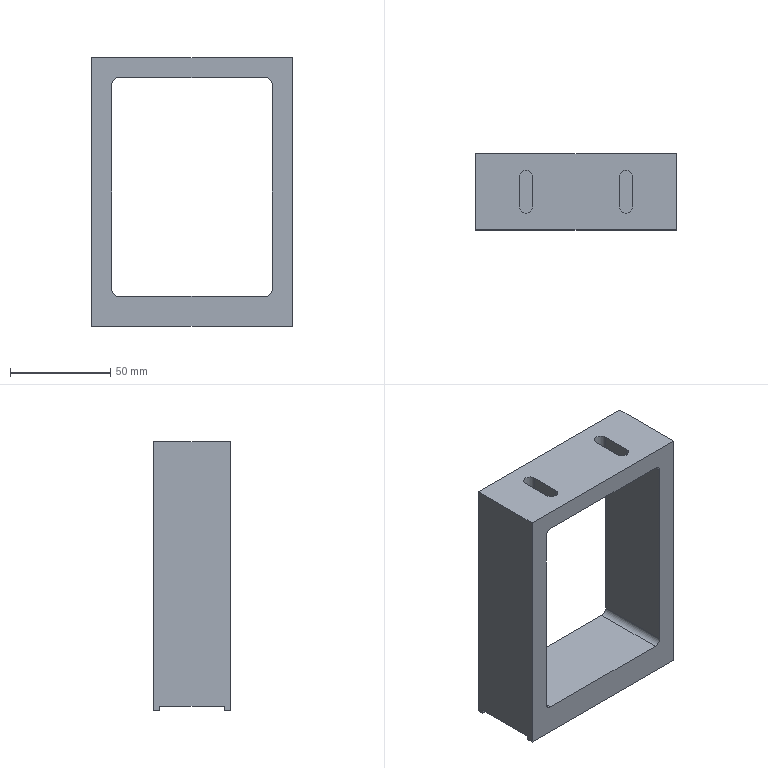Part | NX | features BREP 1 | 1 solid | 42 faces | box 100 x 38 x 134 mm | volume 168763 mm3 | plane 18 | cylinder 16 | cone 8 | commonest cylinder face diameters 3.3 x8 6 x4 6.5 x4
STEP:
#1=CARTESIAN_POINT('',(-38.35,11.,12.1));
#2=VERTEX_POINT('',#1);
#3=CARTESIAN_POINT('',(-41.65,11.,12.1));
#4=VERTEX_POINT('',#3);
#5=CARTESIAN_POINT('',(-40.,11.,12.1));
#6=DIRECTION('',(0.,0.,-1.));
#7=DIRECTION('',(-1.,0.,0.));
#8=AXIS2_PLACEMENT_3D('',#5,#6,#7);
#9=CIRCLE('',#8,1.65);
#10=EDGE_CURVE('',#2,#4,#9,.T.);
#11=ORIENTED_EDGE('',*,*,#10,.F.);
#12=CARTESIAN_POINT('',(-38.35,11.,2.));
#13=VERTEX_POINT('',#12);
#14=CARTESIAN_POINT('',(-38.35,11.,2.));
#15=DIRECTION('',(0.,0.,-1.));
#16=VECTOR('',#15,1000.);
#17=LINE('',#14,#16);
#18=EDGE_CURVE('',#2,#13,#17,.T.);
#19=ORIENTED_EDGE('',*,*,#18,.T.);
#20=CARTESIAN_POINT('',(-41.65,11.,2.));
#21=VERTEX_POINT('',#20);
#22=CARTESIAN_POINT('',(-40.,11.,2.));
#23=DIRECTION('',(0.,0.,-1.));
#24=DIRECTION('',(-1.,0.,0.));
#25=AXIS2_PLACEMENT_3D('',#22,#23,#24);
#26=CIRCLE('',#25,1.65);
#27=EDGE_CURVE('',#13,#21,#26,.T.);
#28=ORIENTED_EDGE('',*,*,#27,.T.);
#29=CARTESIAN_POINT('',(-41.65,11.,2.));
#30=DIRECTION('',(0.,0.,-1.));
#31=VECTOR('',#30,1000.);
#32=LINE('',#29,#31);
#33=EDGE_CURVE('',#4,#21,#32,.T.);
#34=ORIENTED_EDGE('',*,*,#33,.F.);
#35=EDGE_LOOP('',(#11,#19,#28,#34));
#36=FACE_BOUND('',#35,.T.);
#37=CARTESIAN_POINT('',(-40.,11.,2.));
#38=DIRECTION('',(0.,0.,-1.));
#39=DIRECTION('',(-1.,0.,0.));
#40=AXIS2_PLACEMENT_3D('',#37,#38,#39);
#41=CYLINDRICAL_SURFACE('',#40,1.65);
#42=ADVANCED_FACE('',(#36),#41,.F.);
#43=CARTESIAN_POINT('',(-40.,11.,13.091));
#44=VERTEX_POINT('',#43);
#45=CARTESIAN_POINT('',(-41.65,11.,12.1));
#46=DIRECTION('',(-0.8572,0.,-0.515));
#47=VECTOR('',#46,1000.);
#48=LINE('',#45,#47);
#49=EDGE_CURVE('',#44,#4,#48,.T.);
#50=ORIENTED_EDGE('',*,*,#49,.F.);
#51=CARTESIAN_POINT('',(-38.35,11.,12.1));
#52=DIRECTION('',(0.8572,0.,-0.515));
#53=VECTOR('',#52,1000.);
#54=LINE('',#51,#53);
#55=EDGE_CURVE('',#44,#2,#54,.T.);
#56=ORIENTED_EDGE('',*,*,#55,.T.);
#57=ORIENTED_EDGE('',*,*,#10,.T.);
#58=EDGE_LOOP('',(#50,#56,#57));
#59=FACE_BOUND('',#58,.T.);
#60=CARTESIAN_POINT('',(-40.,11.,12.1));
#61=DIRECTION('',(0.,0.,-1.));
#62=DIRECTION('',(-1.,0.,0.));
#63=AXIS2_PLACEMENT_3D('',#60,#61,#62);
#64=CONICAL_SURFACE('',#63,1.65,1.03);
#65=ADVANCED_FACE('',(#59),#64,.F.);
#66=CARTESIAN_POINT('',(-38.35,-11.,12.1));
#67=VERTEX_POINT('',#66);
#68=CARTESIAN_POINT('',(-41.65,-11.,12.1));
#69=VERTEX_POINT('',#68);
#70=CARTESIAN_POINT('',(-40.,-11.,12.1));
#71=DIRECTION('',(0.,0.,-1.));
#72=DIRECTION('',(-1.,0.,0.));
#73=AXIS2_PLACEMENT_3D('',#70,#71,#72);
#74=CIRCLE('',#73,1.65);
#75=EDGE_CURVE('',#67,#69,#74,.T.);
#76=ORIENTED_EDGE('',*,*,#75,.F.);
#77=CARTESIAN_POINT('',(-38.35,-11.,2.));
#78=VERTEX_POINT('',#77);
#79=CARTESIAN_POINT('',(-38.35,-11.,2.));
#80=DIRECTION('',(0.,0.,-1.));
#81=VECTOR('',#80,1000.);
#82=LINE('',#79,#81);
#83=EDGE_CURVE('',#67,#78,#82,.T.);
#84=ORIENTED_EDGE('',*,*,#83,.T.);
#85=CARTESIAN_POINT('',(-41.65,-11.,2.));
#86=VERTEX_POINT('',#85);
#87=CARTESIAN_POINT('',(-40.,-11.,2.));
#88=DIRECTION('',(0.,0.,-1.));
#89=DIRECTION('',(-1.,0.,0.));
#90=AXIS2_PLACEMENT_3D('',#87,#88,#89);
#91=CIRCLE('',#90,1.65);
#92=EDGE_CURVE('',#78,#86,#91,.T.);
#93=ORIENTED_EDGE('',*,*,#92,.T.);
#94=CARTESIAN_POINT('',(-41.65,-11.,2.));
#95=DIRECTION('',(0.,0.,-1.));
#96=VECTOR('',#95,1000.);
#97=LINE('',#94,#96);
#98=EDGE_CURVE('',#69,#86,#97,.T.);
#99=ORIENTED_EDGE('',*,*,#98,.F.);
#100=EDGE_LOOP('',(#76,#84,#93,#99));
#101=FACE_BOUND('',#100,.T.);
#102=CARTESIAN_POINT('',(-40.,-11.,2.));
#103=DIRECTION('',(0.,0.,-1.));
#104=DIRECTION('',(-1.,0.,0.));
#105=AXIS2_PLACEMENT_3D('',#102,#103,#104);
#106=CYLINDRICAL_SURFACE('',#105,1.65);
#107=ADVANCED_FACE('',(#101),#106,.F.);
#108=CARTESIAN_POINT('',(-40.,-11.,13.091));
#109=VERTEX_POINT('',#108);
#110=CARTESIAN_POINT('',(-41.65,-11.,12.1));
#111=DIRECTION('',(-0.8572,0.,-0.515));
#112=VECTOR('',#111,1000.);
#113=LINE('',#110,#112);
#114=EDGE_CURVE('',#109,#69,#113,.T.);
#115=ORIENTED_EDGE('',*,*,#114,.F.);
#116=CARTESIAN_POINT('',(-38.35,-11.,12.1));
#117=DIRECTION('',(0.8572,0.,-0.515));
#118=VECTOR('',#117,1000.);
#119=LINE('',#116,#118);
#120=EDGE_CURVE('',#109,#67,#119,.T.);
#121=ORIENTED_EDGE('',*,*,#120,.T.);
#122=ORIENTED_EDGE('',*,*,#75,.T.);
#123=EDGE_LOOP('',(#115,#121,#122));
#124=FACE_BOUND('',#123,.T.);
#125=CARTESIAN_POINT('',(-40.,-11.,12.1));
#126=DIRECTION('',(0.,0.,-1.));
#127=DIRECTION('',(-1.,0.,0.));
#128=AXIS2_PLACEMENT_3D('',#125,#126,#127);
#129=CONICAL_SURFACE('',#128,1.65,1.03);
#130=ADVANCED_FACE('',(#124),#129,.F.);
#131=CARTESIAN_POINT('',(41.65,11.,12.1));
#132=VERTEX_POINT('',#131);
#133=CARTESIAN_POINT('',(38.35,11.,12.1));
#134=VERTEX_POINT('',#133);
#135=CARTESIAN_POINT('',(40.,11.,12.1));
#136=DIRECTION('',(0.,0.,-1.));
#137=DIRECTION('',(-1.,0.,0.));
#138=AXIS2_PLACEMENT_3D('',#135,#136,#137);
#139=CIRCLE('',#138,1.65);
#140=EDGE_CURVE('',#132,#134,#139,.T.);
#141=ORIENTED_EDGE('',*,*,#140,.F.);
#142=CARTESIAN_POINT('',(41.65,11.,2.));
#143=VERTEX_POINT('',#142);
#144=CARTESIAN_POINT('',(41.65,11.,2.));
#145=DIRECTION('',(0.,0.,-1.));
#146=VECTOR('',#145,1000.);
#147=LINE('',#144,#146);
#148=EDGE_CURVE('',#132,#143,#147,.T.);
#149=ORIENTED_EDGE('',*,*,#148,.T.);
#150=CARTESIAN_POINT('',(38.35,11.,2.));
#151=VERTEX_POINT('',#150);
#152=CARTESIAN_POINT('',(40.,11.,2.));
#153=DIRECTION('',(0.,0.,-1.));
#154=DIRECTION('',(-1.,0.,0.));
#155=AXIS2_PLACEMENT_3D('',#152,#153,#154);
#156=CIRCLE('',#155,1.65);
#157=EDGE_CURVE('',#143,#151,#156,.T.);
#158=ORIENTED_EDGE('',*,*,#157,.T.);
#159=CARTESIAN_POINT('',(38.35,11.,2.));
#160=DIRECTION('',(0.,0.,-1.));
#161=VECTOR('',#160,1000.);
#162=LINE('',#159,#161);
#163=EDGE_CURVE('',#134,#151,#162,.T.);
#164=ORIENTED_EDGE('',*,*,#163,.F.);
#165=EDGE_LOOP('',(#141,#149,#158,#164));
#166=FACE_BOUND('',#165,.T.);
#167=CARTESIAN_POINT('',(40.,11.,2.));
#168=DIRECTION('',(0.,0.,-1.));
#169=DIRECTION('',(-1.,0.,0.));
#170=AXIS2_PLACEMENT_3D('',#167,#168,#169);
#171=CYLINDRICAL_SURFACE('',#170,1.65);
#172=ADVANCED_FACE('',(#166),#171,.F.);
#173=CARTESIAN_POINT('',(40.,11.,13.091));
#174=VERTEX_POINT('',#173);
#175=CARTESIAN_POINT('',(38.35,11.,12.1));
#176=DIRECTION('',(-0.8572,0.,-0.515));
#177=VECTOR('',#176,1000.);
#178=LINE('',#175,#177);
#179=EDGE_CURVE('',#174,#134,#178,.T.);
#180=ORIENTED_EDGE('',*,*,#179,.F.);
#181=CARTESIAN_POINT('',(41.65,11.,12.1));
#182=DIRECTION('',(0.8572,0.,-0.515));
#183=VECTOR('',#182,1000.);
#184=LINE('',#181,#183);
#185=EDGE_CURVE('',#174,#132,#184,.T.);
#186=ORIENTED_EDGE('',*,*,#185,.T.);
#187=ORIENTED_EDGE('',*,*,#140,.T.);
#188=EDGE_LOOP('',(#180,#186,#187));
#189=FACE_BOUND('',#188,.T.);
#190=CARTESIAN_POINT('',(40.,11.,12.1));
#191=DIRECTION('',(0.,0.,-1.));
#192=DIRECTION('',(-1.,0.,0.));
#193=AXIS2_PLACEMENT_3D('',#190,#191,#192);
#194=CONICAL_SURFACE('',#193,1.65,1.03);
#195=ADVANCED_FACE('',(#189),#194,.F.);
#196=CARTESIAN_POINT('',(41.65,-11.,12.1));
#197=VERTEX_POINT('',#196);
#198=CARTESIAN_POINT('',(38.35,-11.,12.1));
#199=VERTEX_POINT('',#198);
#200=CARTESIAN_POINT('',(40.,-11.,12.1));
#201=DIRECTION('',(0.,0.,-1.));
#202=DIRECTION('',(-1.,0.,0.));
#203=AXIS2_PLACEMENT_3D('',#200,#201,#202);
#204=CIRCLE('',#203,1.65);
#205=EDGE_CURVE('',#197,#199,#204,.T.);
#206=ORIENTED_EDGE('',*,*,#205,.F.);
#207=CARTESIAN_POINT('',(41.65,-11.,2.));
#208=VERTEX_POINT('',#207);
#209=CARTESIAN_POINT('',(41.65,-11.,2.));
#210=DIRECTION('',(0.,0.,-1.));
#211=VECTOR('',#210,1000.);
#212=LINE('',#209,#211);
#213=EDGE_CURVE('',#197,#208,#212,.T.);
#214=ORIENTED_EDGE('',*,*,#213,.T.);
#215=CARTESIAN_POINT('',(38.35,-11.,2.));
#216=VERTEX_POINT('',#215);
#217=CARTESIAN_POINT('',(40.,-11.,2.));
#218=DIRECTION('',(0.,0.,-1.));
#219=DIRECTION('',(-1.,0.,0.));
#220=AXIS2_PLACEMENT_3D('',#217,#218,#219);
#221=CIRCLE('',#220,1.65);
#222=EDGE_CURVE('',#208,#216,#221,.T.);
#223=ORIENTED_EDGE('',*,*,#222,.T.);
#224=CARTESIAN_POINT('',(38.35,-11.,2.));
#225=DIRECTION('',(0.,0.,-1.));
#226=VECTOR('',#225,1000.);
#227=LINE('',#224,#226);
#228=EDGE_CURVE('',#199,#216,#227,.T.);
#229=ORIENTED_EDGE('',*,*,#228,.F.);
#230=EDGE_LOOP('',(#206,#214,#223,#229));
#231=FACE_BOUND('',#230,.T.);
#232=CARTESIAN_POINT('',(40.,-11.,2.));
#233=DIRECTION('',(0.,0.,-1.));
#234=DIRECTION('',(-1.,0.,0.));
#235=AXIS2_PLACEMENT_3D('',#232,#233,#234);
#236=CYLINDRICAL_SURFACE('',#235,1.65);
#237=ADVANCED_FACE('',(#231),#236,.F.);
#238=CARTESIAN_POINT('',(40.,-11.,13.091));
#239=VERTEX_POINT('',#238);
#240=CARTESIAN_POINT('',(38.35,-11.,12.1));
#241=DIRECTION('',(-0.8572,0.,-0.515));
#242=VECTOR('',#241,1000.);
#243=LINE('',#240,#242);
#244=EDGE_CURVE('',#239,#199,#243,.T.);
#245=ORIENTED_EDGE('',*,*,#244,.F.);
#246=CARTESIAN_POINT('',(41.65,-11.,12.1));
#247=DIRECTION('',(0.8572,0.,-0.515));
#248=VECTOR('',#247,1000.);
#249=LINE('',#246,#248);
#250=EDGE_CURVE('',#239,#197,#249,.T.);
#251=ORIENTED_EDGE('',*,*,#250,.T.);
#252=ORIENTED_EDGE('',*,*,#205,.T.);
#253=EDGE_LOOP('',(#245,#251,#252));
#254=FACE_BOUND('',#253,.T.);
#255=CARTESIAN_POINT('',(40.,-11.,12.1));
#256=DIRECTION('',(0.,0.,-1.));
#257=DIRECTION('',(-1.,0.,0.));
#258=AXIS2_PLACEMENT_3D('',#255,#256,#257);
#259=CONICAL_SURFACE('',#258,1.65,1.03);
#260=ADVANCED_FACE('',(#254),#259,.F.);
#261=CARTESIAN_POINT('',(-50.,16.,0.));
#262=VERTEX_POINT('',#261);
#263=CARTESIAN_POINT('',(50.,16.,0.));
#264=VERTEX_POINT('',#263);
#265=CARTESIAN_POINT('',(0.,16.,0.));
#266=DIRECTION('',(1.,0.,0.));
#267=VECTOR('',#266,1000.);
#268=LINE('',#265,#267);
#269=EDGE_CURVE('',#262,#264,#268,.T.);
#270=ORIENTED_EDGE('',*,*,#269,.F.);
#271=CARTESIAN_POINT('',(-50.,19.,0.));
#272=VERTEX_POINT('',#271);
#273=CARTESIAN_POINT('',(-50.,-19.,0.));
#274=DIRECTION('',(0.,-1.,0.));
#275=VECTOR('',#274,1000.);
#276=LINE('',#273,#275);
#277=EDGE_CURVE('',#272,#262,#276,.T.);
#278=ORIENTED_EDGE('',*,*,#277,.F.);
#279=CARTESIAN_POINT('',(50.,19.,0.));
#280=VERTEX_POINT('',#279);
#281=CARTESIAN_POINT('',(-50.,19.,0.));
#282=DIRECTION('',(-1.,0.,0.));
#283=VECTOR('',#282,1000.);
#284=LINE('',#281,#283);
#285=EDGE_CURVE('',#280,#272,#284,.T.);
#286=ORIENTED_EDGE('',*,*,#285,.F.);
#287=CARTESIAN_POINT('',(50.,-19.,0.));
#288=DIRECTION('',(0.,1.,0.));
#289=VECTOR('',#288,1000.);
#290=LINE('',#287,#289);
#291=EDGE_CURVE('',#264,#280,#290,.T.);
#292=ORIENTED_EDGE('',*,*,#291,.F.);
#293=EDGE_LOOP('',(#270,#278,#286,#292));
#294=FACE_BOUND('',#293,.T.);
#295=CARTESIAN_POINT('',(0.,0.,0.));
#296=DIRECTION('',(0.,0.,-1.));
#297=DIRECTION('',(0.,-1.,0.));
#298=AXIS2_PLACEMENT_3D('',#295,#296,#297);
#299=PLANE('',#298);
#300=ADVANCED_FACE('',(#294),#299,.T.);
#301=CARTESIAN_POINT('',(50.,16.,2.));
#302=VERTEX_POINT('',#301);
#303=CARTESIAN_POINT('',(50.,-16.,2.));
#304=VERTEX_POINT('',#303);
#305=CARTESIAN_POINT('',(50.,-19.,2.));
#306=DIRECTION('',(0.,-1.,0.));
#307=VECTOR('',#306,1000.);
#308=LINE('',#305,#307);
#309=EDGE_CURVE('',#302,#304,#308,.T.);
#310=ORIENTED_EDGE('',*,*,#309,.F.);
#311=CARTESIAN_POINT('',(50.,16.,134.));
#312=DIRECTION('',(0.,0.,-1.));
#313=VECTOR('',#312,1000.);
#314=LINE('',#311,#313);
#315=EDGE_CURVE('',#302,#264,#314,.T.);
#316=ORIENTED_EDGE('',*,*,#315,.T.);
#317=ORIENTED_EDGE('',*,*,#291,.T.);
#318=CARTESIAN_POINT('',(50.,19.,134.));
#319=VERTEX_POINT('',#318);
#320=CARTESIAN_POINT('',(50.,19.,134.));
#321=DIRECTION('',(0.,0.,-1.));
#322=VECTOR('',#321,1000.);
#323=LINE('',#320,#322);
#324=EDGE_CURVE('',#319,#280,#323,.T.);
#325=ORIENTED_EDGE('',*,*,#324,.F.);
#326=CARTESIAN_POINT('',(50.,-19.,134.));
#327=VERTEX_POINT('',#326);
#328=CARTESIAN_POINT('',(50.,-19.,134.));
#329=DIRECTION('',(0.,1.,0.));
#330=VECTOR('',#329,1000.);
#331=LINE('',#328,#330);
#332=EDGE_CURVE('',#327,#319,#331,.T.);
#333=ORIENTED_EDGE('',*,*,#332,.F.);
#334=CARTESIAN_POINT('',(50.,-19.,0.));
#335=VERTEX_POINT('',#334);
#336=CARTESIAN_POINT('',(50.,-19.,134.));
#337=DIRECTION('',(0.,0.,-1.));
#338=VECTOR('',#337,1000.);
#339=LINE('',#336,#338);
#340=EDGE_CURVE('',#327,#335,#339,.T.);
#341=ORIENTED_EDGE('',*,*,#340,.T.);
#342=CARTESIAN_POINT('',(50.,-16.,0.));
#343=VERTEX_POINT('',#342);
#344=CARTESIAN_POINT('',(50.,-19.,0.));
#345=DIRECTION('',(0.,1.,0.));
#346=VECTOR('',#345,1000.);
#347=LINE('',#344,#346);
#348=EDGE_CURVE('',#335,#343,#347,.T.);
#349=ORIENTED_EDGE('',*,*,#348,.T.);
#350=CARTESIAN_POINT('',(50.,-16.,134.));
#351=DIRECTION('',(0.,0.,1.));
#352=VECTOR('',#351,1000.);
#353=LINE('',#350,#352);
#354=EDGE_CURVE('',#343,#304,#353,.T.);
#355=ORIENTED_EDGE('',*,*,#354,.T.);
#356=EDGE_LOOP('',(#310,#316,#317,#325,#333,#341,#349,#355));
#357=FACE_BOUND('',#356,.T.);
#358=CARTESIAN_POINT('',(50.,-19.,134.));
#359=DIRECTION('',(-1.,0.,0.));
#360=DIRECTION('',(0.,0.,1.));
#361=AXIS2_PLACEMENT_3D('',#358,#359,#360);
#362=PLANE('',#361);
#363=ADVANCED_FACE('',(#357),#362,.F.);
#364=ORIENTED_EDGE('',*,*,#285,.T.);
#365=CARTESIAN_POINT('',(-50.,19.,134.));
#366=VERTEX_POINT('',#365);
#367=CARTESIAN_POINT('',(-50.,19.,134.));
#368=DIRECTION('',(0.,0.,-1.));
#369=VECTOR('',#368,1000.);
#370=LINE('',#367,#369);
#371=EDGE_CURVE('',#366,#272,#370,.T.);
#372=ORIENTED_EDGE('',*,*,#371,.F.);
#373=CARTESIAN_POINT('',(-50.,19.,134.));
#374=DIRECTION('',(-1.,0.,0.));
#375=VECTOR('',#374,1000.);
#376=LINE('',#373,#375);
#377=EDGE_CURVE('',#319,#366,#376,.T.);
#378=ORIENTED_EDGE('',*,*,#377,.F.);
#379=ORIENTED_EDGE('',*,*,#324,.T.);
#380=EDGE_LOOP('',(#364,#372,#378,#379));
#381=FACE_BOUND('',#380,.T.);
#382=CARTESIAN_POINT('',(40.,19.,18.));
#383=VERTEX_POINT('',#382);
#384=CARTESIAN_POINT('',(40.,19.,121.));
#385=VERTEX_POINT('',#384);
#386=CARTESIAN_POINT('',(40.,19.,124.));
#387=DIRECTION('',(0.,0.,1.));
#388=VECTOR('',#387,1000.);
#389=LINE('',#386,#388);
#390=EDGE_CURVE('',#383,#385,#389,.T.);
#391=ORIENTED_EDGE('',*,*,#390,.T.);
#392=CARTESIAN_POINT('',(37.,19.,124.));
#393=VERTEX_POINT('',#392);
#394=CARTESIAN_POINT('',(37.,19.,121.));
#395=DIRECTION('',(0.,-1.,0.));
#396=DIRECTION('',(0.,0.,-1.));
#397=AXIS2_PLACEMENT_3D('',#394,#395,#396);
#398=CIRCLE('',#397,3.);
#399=EDGE_CURVE('',#385,#393,#398,.T.);
#400=ORIENTED_EDGE('',*,*,#399,.T.);
#401=CARTESIAN_POINT('',(-37.,19.,124.));
#402=VERTEX_POINT('',#401);
#403=CARTESIAN_POINT('',(40.,19.,124.));
#404=DIRECTION('',(-1.,0.,0.));
#405=VECTOR('',#404,1000.);
#406=LINE('',#403,#405);
#407=EDGE_CURVE('',#393,#402,#406,.T.);
#408=ORIENTED_EDGE('',*,*,#407,.T.);
#409=CARTESIAN_POINT('',(-40.,19.,121.));
#410=VERTEX_POINT('',#409);
#411=CARTESIAN_POINT('',(-37.,19.,121.));
#412=DIRECTION('',(0.,-1.,0.));
#413=DIRECTION('',(0.,0.,-1.));
#414=AXIS2_PLACEMENT_3D('',#411,#412,#413);
#415=CIRCLE('',#414,3.);
#416=EDGE_CURVE('',#402,#410,#415,.T.);
#417=ORIENTED_EDGE('',*,*,#416,.T.);
#418=CARTESIAN_POINT('',(-40.,19.,18.));
#419=VERTEX_POINT('',#418);
#420=CARTESIAN_POINT('',(-40.,19.,124.));
#421=DIRECTION('',(0.,0.,-1.));
#422=VECTOR('',#421,1000.);
#423=LINE('',#420,#422);
#424=EDGE_CURVE('',#410,#419,#423,.T.);
#425=ORIENTED_EDGE('',*,*,#424,.T.);
#426=CARTESIAN_POINT('',(-37.,19.,15.));
#427=VERTEX_POINT('',#426);
#428=CARTESIAN_POINT('',(-37.,19.,18.));
#429=DIRECTION('',(0.,-1.,0.));
#430=DIRECTION('',(0.,0.,-1.));
#431=AXIS2_PLACEMENT_3D('',#428,#429,#430);
#432=CIRCLE('',#431,3.);
#433=EDGE_CURVE('',#419,#427,#432,.T.);
#434=ORIENTED_EDGE('',*,*,#433,.T.);
#435=CARTESIAN_POINT('',(37.,19.,15.));
#436=VERTEX_POINT('',#435);
#437=CARTESIAN_POINT('',(40.,19.,15.));
#438=DIRECTION('',(1.,0.,0.));
#439=VECTOR('',#438,1000.);
#440=LINE('',#437,#439);
#441=EDGE_CURVE('',#427,#436,#440,.T.);
#442=ORIENTED_EDGE('',*,*,#441,.T.);
#443=CARTESIAN_POINT('',(37.,19.,18.));
#444=DIRECTION('',(0.,-1.,0.));
#445=DIRECTION('',(0.,0.,-1.));
#446=AXIS2_PLACEMENT_3D('',#443,#444,#445);
#447=CIRCLE('',#446,3.);
#448=EDGE_CURVE('',#436,#383,#447,.T.);
#449=ORIENTED_EDGE('',*,*,#448,.T.);
#450=EDGE_LOOP('',(#391,#400,#408,#417,#425,#434,#442,#449));
#451=FACE_BOUND('',#450,.T.);
#452=CARTESIAN_POINT('',(-50.,19.,134.));
#453=DIRECTION('',(0.,-1.,0.));
#454=DIRECTION('',(0.,0.,-1.));
#455=AXIS2_PLACEMENT_3D('',#452,#453,#454);
#456=PLANE('',#455);
#457=ADVANCED_FACE('',(#381,#451),#456,.F.);
#458=ORIENTED_EDGE('',*,*,#277,.T.);
#459=CARTESIAN_POINT('',(-50.,16.,2.));
#460=VERTEX_POINT('',#459);
#461=CARTESIAN_POINT('',(-50.,16.,134.));
#462=DIRECTION('',(0.,0.,1.));
#463=VECTOR('',#462,1000.);
#464=LINE('',#461,#463);
#465=EDGE_CURVE('',#262,#460,#464,.T.);
#466=ORIENTED_EDGE('',*,*,#465,.T.);
#467=CARTESIAN_POINT('',(-50.,-16.,2.));
#468=VERTEX_POINT('',#467);
#469=CARTESIAN_POINT('',(-50.,-19.,2.));
#470=DIRECTION('',(0.,1.,0.));
#471=VECTOR('',#470,1000.);
#472=LINE('',#469,#471);
#473=EDGE_CURVE('',#468,#460,#472,.T.);
#474=ORIENTED_EDGE('',*,*,#473,.F.);
#475=CARTESIAN_POINT('',(-50.,-16.,0.));
#476=VERTEX_POINT('',#475);
#477=CARTESIAN_POINT('',(-50.,-16.,134.));
#478=DIRECTION('',(0.,0.,-1.));
#479=VECTOR('',#478,1000.);
#480=LINE('',#477,#479);
#481=EDGE_CURVE('',#468,#476,#480,.T.);
#482=ORIENTED_EDGE('',*,*,#481,.T.);
#483=CARTESIAN_POINT('',(-50.,-19.,0.));
#484=VERTEX_POINT('',#483);
#485=CARTESIAN_POINT('',(-50.,-19.,0.));
#486=DIRECTION('',(0.,-1.,0.));
#487=VECTOR('',#486,1000.);
#488=LINE('',#485,#487);
#489=EDGE_CURVE('',#476,#484,#488,.T.);
#490=ORIENTED_EDGE('',*,*,#489,.T.);
#491=CARTESIAN_POINT('',(-50.,-19.,134.));
#492=VERTEX_POINT('',#491);
#493=CARTESIAN_POINT('',(-50.,-19.,134.));
#494=DIRECTION('',(0.,0.,-1.));
#495=VECTOR('',#494,1000.);
#496=LINE('',#493,#495);
#497=EDGE_CURVE('',#492,#484,#496,.T.);
#498=ORIENTED_EDGE('',*,*,#497,.F.);
#499=CARTESIAN_POINT('',(-50.,-19.,134.));
#500=DIRECTION('',(0.,-1.,0.));
#501=VECTOR('',#500,1000.);
#502=LINE('',#499,#501);
#503=EDGE_CURVE('',#366,#492,#502,.T.);
#504=ORIENTED_EDGE('',*,*,#503,.F.);
#505=ORIENTED_EDGE('',*,*,#371,.T.);
#506=EDGE_LOOP('',(#458,#466,#474,#482,#490,#498,#504,#505));
#507=FACE_BOUND('',#506,.T.);
#508=CARTESIAN_POINT('',(-50.,-19.,134.));
#509=DIRECTION('',(1.,0.,0.));
#510=DIRECTION('',(0.,1.,0.));
#511=AXIS2_PLACEMENT_3D('',#508,#509,#510);
#512=PLANE('',#511);
#513=ADVANCED_FACE('',(#507),#512,.F.);
#514=CARTESIAN_POINT('',(-50.,-19.,0.));
#515=DIRECTION('',(1.,0.,0.));
#516=VECTOR('',#515,1000.);
#517=LINE('',#514,#516);
#518=EDGE_CURVE('',#484,#335,#517,.T.);
#519=ORIENTED_EDGE('',*,*,#518,.T.);
#520=ORIENTED_EDGE('',*,*,#340,.F.);
#521=CARTESIAN_POINT('',(-50.,-19.,134.));
#522=DIRECTION('',(1.,0.,0.));
#523=VECTOR('',#522,1000.);
#524=LINE('',#521,#523);
#525=EDGE_CURVE('',#492,#327,#524,.T.);
#526=ORIENTED_EDGE('',*,*,#525,.F.);
#527=ORIENTED_EDGE('',*,*,#497,.T.);
#528=EDGE_LOOP('',(#519,#520,#526,#527));
#529=FACE_BOUND('',#528,.T.);
#530=CARTESIAN_POINT('',(-37.,-19.,15.));
#531=VERTEX_POINT('',#530);
#532=CARTESIAN_POINT('',(37.,-19.,15.));
#533=VERTEX_POINT('',#532);
#534=CARTESIAN_POINT('',(40.,-19.,15.));
#535=DIRECTION('',(1.,0.,0.));
#536=VECTOR('',#535,1000.);
#537=LINE('',#534,#536);
#538=EDGE_CURVE('',#531,#533,#537,.T.);
#539=ORIENTED_EDGE('',*,*,#538,.F.);
#540=CARTESIAN_POINT('',(-40.,-19.,18.));
#541=VERTEX_POINT('',#540);
#542=CARTESIAN_POINT('',(-37.,-19.,18.));
#543=DIRECTION('',(0.,1.,0.));
#544=DIRECTION('',(0.,0.,1.));
#545=AXIS2_PLACEMENT_3D('',#542,#543,#544);
#546=CIRCLE('',#545,3.);
#547=EDGE_CURVE('',#531,#541,#546,.T.);
#548=ORIENTED_EDGE('',*,*,#547,.T.);
#549=CARTESIAN_POINT('',(-40.,-19.,121.));
#550=VERTEX_POINT('',#549);
#551=CARTESIAN_POINT('',(-40.,-19.,124.));
#552=DIRECTION('',(0.,0.,-1.));
#553=VECTOR('',#552,1000.);
#554=LINE('',#551,#553);
#555=EDGE_CURVE('',#550,#541,#554,.T.);
#556=ORIENTED_EDGE('',*,*,#555,.F.);
#557=CARTESIAN_POINT('',(-37.,-19.,124.));
#558=VERTEX_POINT('',#557);
#559=CARTESIAN_POINT('',(-37.,-19.,121.));
#560=DIRECTION('',(0.,1.,0.));
#561=DIRECTION('',(0.,0.,1.));
#562=AXIS2_PLACEMENT_3D('',#559,#560,#561);
#563=CIRCLE('',#562,3.);
#564=EDGE_CURVE('',#550,#558,#563,.T.);
#565=ORIENTED_EDGE('',*,*,#564,.T.);
#566=CARTESIAN_POINT('',(37.,-19.,124.));
#567=VERTEX_POINT('',#566);
#568=CARTESIAN_POINT('',(40.,-19.,124.));
#569=DIRECTION('',(-1.,0.,0.));
#570=VECTOR('',#569,1000.);
#571=LINE('',#568,#570);
#572=EDGE_CURVE('',#567,#558,#571,.T.);
#573=ORIENTED_EDGE('',*,*,#572,.F.);
#574=CARTESIAN_POINT('',(40.,-19.,121.));
#575=VERTEX_POINT('',#574);
#576=CARTESIAN_POINT('',(37.,-19.,121.));
#577=DIRECTION('',(0.,1.,0.));
#578=DIRECTION('',(0.,0.,1.));
#579=AXIS2_PLACEMENT_3D('',#576,#577,#578);
#580=CIRCLE('',#579,3.);
#581=EDGE_CURVE('',#567,#575,#580,.T.);
#582=ORIENTED_EDGE('',*,*,#581,.T.);
#583=CARTESIAN_POINT('',(40.,-19.,18.));
#584=VERTEX_POINT('',#583);
#585=CARTESIAN_POINT('',(40.,-19.,124.));
#586=DIRECTION('',(0.,0.,1.));
#587=VECTOR('',#586,1000.);
#588=LINE('',#585,#587);
#589=EDGE_CURVE('',#584,#575,#588,.T.);
#590=ORIENTED_EDGE('',*,*,#589,.F.);
#591=CARTESIAN_POINT('',(37.,-19.,18.));
#592=DIRECTION('',(0.,1.,0.));
#593=DIRECTION('',(0.,0.,1.));
#594=AXIS2_PLACEMENT_3D('',#591,#592,#593);
#595=CIRCLE('',#594,3.);
#596=EDGE_CURVE('',#584,#533,#595,.T.);
#597=ORIENTED_EDGE('',*,*,#596,.T.);
#598=EDGE_LOOP('',(#539,#548,#556,#565,#573,#582,#590,#597));
#599=FACE_BOUND('',#598,.T.);
#600=CARTESIAN_POINT('',(-50.,-19.,134.));
#601=DIRECTION('',(0.,1.,0.));
#602=DIRECTION('',(1.,0.,0.));
#603=AXIS2_PLACEMENT_3D('',#600,#601,#602);
#604=PLANE('',#603);
#605=ADVANCED_FACE('',(#529,#599),#604,.F.);
#606=ORIENTED_EDGE('',*,*,#332,.T.);
#607=ORIENTED_EDGE('',*,*,#377,.T.);
#608=ORIENTED_EDGE('',*,*,#503,.T.);
#609=ORIENTED_EDGE('',*,*,#525,.T.);
#610=EDGE_LOOP('',(#606,#607,#608,#609));
#611=FACE_BOUND('',#610,.T.);
#612=CARTESIAN_POINT('',(28.25,7.5,134.));
#613=VERTEX_POINT('',#612);
#614=CARTESIAN_POINT('',(28.25,-7.5,134.));
#615=VERTEX_POINT('',#614);
#616=CARTESIAN_POINT('',(28.25,-7.5,134.));
#617=DIRECTION('',(0.,-1.,0.));
#618=VECTOR('',#617,1000.);
#619=LINE('',#616,#618);
#620=EDGE_CURVE('',#613,#615,#619,.T.);
#621=ORIENTED_EDGE('',*,*,#620,.T.);
#622=CARTESIAN_POINT('',(21.75,-7.5,134.));
#623=VERTEX_POINT('',#622);
#624=CARTESIAN_POINT('',(25.,-7.5,134.));
#625=DIRECTION('',(0.,0.,-1.));
#626=DIRECTION('',(-1.,0.,0.));
#627=AXIS2_PLACEMENT_3D('',#624,#625,#626);
#628=CIRCLE('',#627,3.25);
#629=EDGE_CURVE('',#615,#623,#628,.T.);
#630=ORIENTED_EDGE('',*,*,#629,.T.);
#631=CARTESIAN_POINT('',(21.75,7.5,134.));
#632=VERTEX_POINT('',#631);
#633=CARTESIAN_POINT('',(21.75,-7.5,134.));
#634=DIRECTION('',(0.,1.,0.));
#635=VECTOR('',#634,1000.);
#636=LINE('',#633,#635);
#637=EDGE_CURVE('',#623,#632,#636,.T.);
#638=ORIENTED_EDGE('',*,*,#637,.T.);
#639=CARTESIAN_POINT('',(25.,7.5,134.));
#640=DIRECTION('',(0.,0.,-1.));
#641=DIRECTION('',(-1.,0.,0.));
#642=AXIS2_PLACEMENT_3D('',#639,#640,#641);
#643=CIRCLE('',#642,3.25);
#644=EDGE_CURVE('',#632,#613,#643,.T.);
#645=ORIENTED_EDGE('',*,*,#644,.T.);
#646=EDGE_LOOP('',(#621,#630,#638,#645));
#647=FACE_BOUND('',#646,.T.);
#648=CARTESIAN_POINT('',(-21.75,7.5,134.));
#649=VERTEX_POINT('',#648);
#650=CARTESIAN_POINT('',(-21.75,-7.5,134.));
#651=VERTEX_POINT('',#650);
#652=CARTESIAN_POINT('',(-21.75,-7.5,134.));
#653=DIRECTION('',(0.,-1.,0.));
#654=VECTOR('',#653,1000.);
#655=LINE('',#652,#654);
#656=EDGE_CURVE('',#649,#651,#655,.T.);
#657=ORIENTED_EDGE('',*,*,#656,.T.);
#658=CARTESIAN_POINT('',(-28.25,-7.5,134.));
#659=VERTEX_POINT('',#658);
#660=CARTESIAN_POINT('',(-25.,-7.5,134.));
#661=DIRECTION('',(0.,0.,-1.));
#662=DIRECTION('',(-1.,0.,0.));
#663=AXIS2_PLACEMENT_3D('',#660,#661,#662);
#664=CIRCLE('',#663,3.25);
#665=EDGE_CURVE('',#651,#659,#664,.T.);
#666=ORIENTED_EDGE('',*,*,#665,.T.);
#667=CARTESIAN_POINT('',(-28.25,7.5,134.));
#668=VERTEX_POINT('',#667);
#669=CARTESIAN_POINT('',(-28.25,-7.5,134.));
#670=DIRECTION('',(0.,1.,0.));
#671=VECTOR('',#670,1000.);
#672=LINE('',#669,#671);
#673=EDGE_CURVE('',#659,#668,#672,.T.);
#674=ORIENTED_EDGE('',*,*,#673,.T.);
#675=CARTESIAN_POINT('',(-25.,7.5,134.));
#676=DIRECTION('',(0.,0.,-1.));
#677=DIRECTION('',(-1.,0.,0.));
#678=AXIS2_PLACEMENT_3D('',#675,#676,#677);
#679=CIRCLE('',#678,3.25);
#680=EDGE_CURVE('',#668,#649,#679,.T.);
#681=ORIENTED_EDGE('',*,*,#680,.T.);
#682=EDGE_LOOP('',(#657,#666,#674,#681));
#683=FACE_BOUND('',#682,.T.);
#684=CARTESIAN_POINT('',(0.,0.,134.));
#685=DIRECTION('',(0.,0.,-1.));
#686=DIRECTION('',(0.,-1.,0.));
#687=AXIS2_PLACEMENT_3D('',#684,#685,#686);
#688=PLANE('',#687);
#689=ADVANCED_FACE('',(#611,#647,#683),#688,.F.);
#690=CARTESIAN_POINT('',(0.,-16.,0.));
#691=DIRECTION('',(-1.,0.,0.));
#692=VECTOR('',#691,1000.);
#693=LINE('',#690,#692);
#694=EDGE_CURVE('',#343,#476,#693,.T.);
#695=ORIENTED_EDGE('',*,*,#694,.F.);
#696=ORIENTED_EDGE('',*,*,#348,.F.);
#697=ORIENTED_EDGE('',*,*,#518,.F.);
#698=ORIENTED_EDGE('',*,*,#489,.F.);
#699=EDGE_LOOP('',(#695,#696,#697,#698));
#700=FACE_BOUND('',#699,.T.);
#701=CARTESIAN_POINT('',(0.,0.,0.));
#702=DIRECTION('',(0.,0.,-1.));
#703=DIRECTION('',(0.,-1.,0.));
#704=AXIS2_PLACEMENT_3D('',#701,#702,#703);
#705=PLANE('',#704);
#706=ADVANCED_FACE('',(#700),#705,.T.);
#707=ORIENTED_EDGE('',*,*,#309,.T.);
#708=CARTESIAN_POINT('',(-83.786,-16.,2.));
#709=DIRECTION('',(-1.,0.,0.));
#710=VECTOR('',#709,1000.);
#711=LINE('',#708,#710);
#712=EDGE_CURVE('',#304,#468,#711,.T.);
#713=ORIENTED_EDGE('',*,*,#712,.T.);
#714=ORIENTED_EDGE('',*,*,#473,.T.);
#715=CARTESIAN_POINT('',(-83.786,16.,2.));
#716=DIRECTION('',(1.,0.,0.));
#717=VECTOR('',#716,1000.);
#718=LINE('',#715,#717);
#719=EDGE_CURVE('',#460,#302,#718,.T.);
#720=ORIENTED_EDGE('',*,*,#719,.T.);
#721=EDGE_LOOP('',(#707,#713,#714,#720));
#722=FACE_BOUND('',#721,.T.);
#723=CARTESIAN_POINT('',(-40.,11.,2.));
#724=DIRECTION('',(0.,0.,-1.));
#725=DIRECTION('',(-1.,0.,0.));
#726=AXIS2_PLACEMENT_3D('',#723,#724,#725);
#727=CIRCLE('',#726,1.65);
#728=EDGE_CURVE('',#21,#13,#727,.T.);
#729=ORIENTED_EDGE('',*,*,#728,.F.);
#730=ORIENTED_EDGE('',*,*,#27,.F.);
#731=EDGE_LOOP('',(#729,#730));
#732=FACE_BOUND('',#731,.T.);
#733=CARTESIAN_POINT('',(-40.,-11.,2.));
#734=DIRECTION('',(0.,0.,-1.));
#735=DIRECTION('',(-1.,0.,0.));
#736=AXIS2_PLACEMENT_3D('',#733,#734,#735);
#737=CIRCLE('',#736,1.65);
#738=EDGE_CURVE('',#86,#78,#737,.T.);
#739=ORIENTED_EDGE('',*,*,#738,.F.);
#740=ORIENTED_EDGE('',*,*,#92,.F.);
#741=EDGE_LOOP('',(#739,#740));
#742=FACE_BOUND('',#741,.T.);
#743=CARTESIAN_POINT('',(40.,11.,2.));
#744=DIRECTION('',(0.,0.,-1.));
#745=DIRECTION('',(-1.,0.,0.));
#746=AXIS2_PLACEMENT_3D('',#743,#744,#745);
#747=CIRCLE('',#746,1.65);
#748=EDGE_CURVE('',#151,#143,#747,.T.);
#749=ORIENTED_EDGE('',*,*,#748,.F.);
#750=ORIENTED_EDGE('',*,*,#157,.F.);
#751=EDGE_LOOP('',(#749,#750));
#752=FACE_BOUND('',#751,.T.);
#753=CARTESIAN_POINT('',(40.,-11.,2.));
#754=DIRECTION('',(0.,0.,-1.));
#755=DIRECTION('',(-1.,0.,0.));
#756=AXIS2_PLACEMENT_3D('',#753,#754,#755);
#757=CIRCLE('',#756,1.65);
#758=EDGE_CURVE('',#216,#208,#757,.T.);
#759=ORIENTED_EDGE('',*,*,#758,.F.);
#760=ORIENTED_EDGE('',*,*,#222,.F.);
#761=EDGE_LOOP('',(#759,#760));
#762=FACE_BOUND('',#761,.T.);
#763=CARTESIAN_POINT('',(0.,0.,2.));
#764=DIRECTION('',(0.,0.,-1.));
#765=DIRECTION('',(0.,-1.,0.));
#766=AXIS2_PLACEMENT_3D('',#763,#764,#765);
#767=PLANE('',#766);
#768=ADVANCED_FACE('',(#722,#732,#742,#752,#762),#767,.T.);
#769=ORIENTED_EDGE('',*,*,#719,.F.);
#770=ORIENTED_EDGE('',*,*,#465,.F.);
#771=ORIENTED_EDGE('',*,*,#269,.T.);
#772=ORIENTED_EDGE('',*,*,#315,.F.);
#773=EDGE_LOOP('',(#769,#770,#771,#772));
#774=FACE_BOUND('',#773,.T.);
#775=CARTESIAN_POINT('',(-83.786,16.,2.));
#776=DIRECTION('',(0.,1.,0.));
#777=DIRECTION('',(1.,0.,0.));
#778=AXIS2_PLACEMENT_3D('',#775,#776,#777);
#779=PLANE('',#778);
#780=ADVANCED_FACE('',(#774),#779,.F.);
#781=ORIENTED_EDGE('',*,*,#694,.T.);
#782=ORIENTED_EDGE('',*,*,#481,.F.);
#783=ORIENTED_EDGE('',*,*,#712,.F.);
#784=ORIENTED_EDGE('',*,*,#354,.F.);
#785=EDGE_LOOP('',(#781,#782,#783,#784));
#786=FACE_BOUND('',#785,.T.);
#787=CARTESIAN_POINT('',(-83.786,-16.,2.));
#788=DIRECTION('',(0.,-1.,0.));
#789=DIRECTION('',(-1.,0.,0.));
#790=AXIS2_PLACEMENT_3D('',#787,#788,#789);
#791=PLANE('',#790);
#792=ADVANCED_FACE('',(#786),#791,.F.);
#793=ORIENTED_EDGE('',*,*,#424,.F.);
#794=CARTESIAN_POINT('',(-40.,-19.,121.));
#795=DIRECTION('',(0.,-1.,0.));
#796=VECTOR('',#795,1000.);
#797=LINE('',#794,#796);
#798=EDGE_CURVE('',#410,#550,#797,.T.);
#799=ORIENTED_EDGE('',*,*,#798,.T.);
#800=ORIENTED_EDGE('',*,*,#555,.T.);
#801=CARTESIAN_POINT('',(-40.,19.,18.));
#802=DIRECTION('',(0.,1.,0.));
#803=VECTOR('',#802,1000.);
#804=LINE('',#801,#803);
#805=EDGE_CURVE('',#541,#419,#804,.T.);
#806=ORIENTED_EDGE('',*,*,#805,.T.);
#807=EDGE_LOOP('',(#793,#799,#800,#806));
#808=FACE_BOUND('',#807,.T.);
#809=CARTESIAN_POINT('',(-40.,19.,124.));
#810=DIRECTION('',(-1.,0.,0.));
#811=DIRECTION('',(0.,0.,1.));
#812=AXIS2_PLACEMENT_3D('',#809,#810,#811);
#813=PLANE('',#812);
#814=ADVANCED_FACE('',(#808),#813,.F.);
#815=ORIENTED_EDGE('',*,*,#407,.F.);
#816=CARTESIAN_POINT('',(37.,-19.,124.));
#817=DIRECTION('',(0.,-1.,0.));
#818=VECTOR('',#817,1000.);
#819=LINE('',#816,#818);
#820=EDGE_CURVE('',#393,#567,#819,.T.);
#821=ORIENTED_EDGE('',*,*,#820,.T.);
#822=ORIENTED_EDGE('',*,*,#572,.T.);
#823=CARTESIAN_POINT('',(-37.,19.,124.));
#824=DIRECTION('',(0.,1.,0.));
#825=VECTOR('',#824,1000.);
#826=LINE('',#823,#825);
#827=EDGE_CURVE('',#558,#402,#826,.T.);
#828=ORIENTED_EDGE('',*,*,#827,.T.);
#829=EDGE_LOOP('',(#815,#821,#822,#828));
#830=FACE_BOUND('',#829,.T.);
#831=CARTESIAN_POINT('',(21.75,-7.5,124.));
#832=VERTEX_POINT('',#831);
#833=CARTESIAN_POINT('',(21.75,7.5,124.));
#834=VERTEX_POINT('',#833);
#835=CARTESIAN_POINT('',(21.75,-7.5,124.));
#836=DIRECTION('',(0.,1.,0.));
#837=VECTOR('',#836,1000.);
#838=LINE('',#835,#837);
#839=EDGE_CURVE('',#832,#834,#838,.T.);
#840=ORIENTED_EDGE('',*,*,#839,.F.);
#841=CARTESIAN_POINT('',(28.25,-7.5,124.));
#842=VERTEX_POINT('',#841);
#843=CARTESIAN_POINT('',(25.,-7.5,124.));
#844=DIRECTION('',(0.,0.,-1.));
#845=DIRECTION('',(-1.,0.,0.));
#846=AXIS2_PLACEMENT_3D('',#843,#844,#845);
#847=CIRCLE('',#846,3.25);
#848=EDGE_CURVE('',#842,#832,#847,.T.);
#849=ORIENTED_EDGE('',*,*,#848,.F.);
#850=CARTESIAN_POINT('',(28.25,7.5,124.));
#851=VERTEX_POINT('',#850);
#852=CARTESIAN_POINT('',(28.25,-7.5,124.));
#853=DIRECTION('',(0.,-1.,0.));
#854=VECTOR('',#853,1000.);
#855=LINE('',#852,#854);
#856=EDGE_CURVE('',#851,#842,#855,.T.);
#857=ORIENTED_EDGE('',*,*,#856,.F.);
#858=CARTESIAN_POINT('',(25.,7.5,124.));
#859=DIRECTION('',(0.,0.,-1.));
#860=DIRECTION('',(-1.,0.,0.));
#861=AXIS2_PLACEMENT_3D('',#858,#859,#860);
#862=CIRCLE('',#861,3.25);
#863=EDGE_CURVE('',#834,#851,#862,.T.);
#864=ORIENTED_EDGE('',*,*,#863,.F.);
#865=EDGE_LOOP('',(#840,#849,#857,#864));
#866=FACE_BOUND('',#865,.T.);
#867=CARTESIAN_POINT('',(-28.25,-7.5,124.));
#868=VERTEX_POINT('',#867);
#869=CARTESIAN_POINT('',(-28.25,7.5,124.));
#870=VERTEX_POINT('',#869);
#871=CARTESIAN_POINT('',(-28.25,-7.5,124.));
#872=DIRECTION('',(0.,1.,0.));
#873=VECTOR('',#872,1000.);
#874=LINE('',#871,#873);
#875=EDGE_CURVE('',#868,#870,#874,.T.);
#876=ORIENTED_EDGE('',*,*,#875,.F.);
#877=CARTESIAN_POINT('',(-21.75,-7.5,124.));
#878=VERTEX_POINT('',#877);
#879=CARTESIAN_POINT('',(-25.,-7.5,124.));
#880=DIRECTION('',(0.,0.,-1.));
#881=DIRECTION('',(-1.,0.,0.));
#882=AXIS2_PLACEMENT_3D('',#879,#880,#881);
#883=CIRCLE('',#882,3.25);
#884=EDGE_CURVE('',#878,#868,#883,.T.);
#885=ORIENTED_EDGE('',*,*,#884,.F.);
#886=CARTESIAN_POINT('',(-21.75,7.5,124.));
#887=VERTEX_POINT('',#886);
#888=CARTESIAN_POINT('',(-21.75,-7.5,124.));
#889=DIRECTION('',(0.,-1.,0.));
#890=VECTOR('',#889,1000.);
#891=LINE('',#888,#890);
#892=EDGE_CURVE('',#887,#878,#891,.T.);
#893=ORIENTED_EDGE('',*,*,#892,.F.);
#894=CARTESIAN_POINT('',(-25.,7.5,124.));
#895=DIRECTION('',(0.,0.,-1.));
#896=DIRECTION('',(-1.,0.,0.));
#897=AXIS2_PLACEMENT_3D('',#894,#895,#896);
#898=CIRCLE('',#897,3.25);
#899=EDGE_CURVE('',#870,#887,#898,.T.);
#900=ORIENTED_EDGE('',*,*,#899,.F.);
#901=EDGE_LOOP('',(#876,#885,#893,#900));
#902=FACE_BOUND('',#901,.T.);
#903=CARTESIAN_POINT('',(40.,19.,124.));
#904=DIRECTION('',(0.,0.,1.));
#905=DIRECTION('',(1.,0.,0.));
#906=AXIS2_PLACEMENT_3D('',#903,#904,#905);
#907=PLANE('',#906);
#908=ADVANCED_FACE('',(#830,#866,#902),#907,.F.);
#909=ORIENTED_EDGE('',*,*,#589,.T.);
#910=CARTESIAN_POINT('',(40.,19.,121.));
#911=DIRECTION('',(0.,1.,0.));
#912=VECTOR('',#911,1000.);
#913=LINE('',#910,#912);
#914=EDGE_CURVE('',#575,#385,#913,.T.);
#915=ORIENTED_EDGE('',*,*,#914,.T.);
#916=ORIENTED_EDGE('',*,*,#390,.F.);
#917=CARTESIAN_POINT('',(40.,-19.,18.));
#918=DIRECTION('',(0.,-1.,0.));
#919=VECTOR('',#918,1000.);
#920=LINE('',#917,#919);
#921=EDGE_CURVE('',#383,#584,#920,.T.);
#922=ORIENTED_EDGE('',*,*,#921,.T.);
#923=EDGE_LOOP('',(#909,#915,#916,#922));
#924=FACE_BOUND('',#923,.T.);
#925=CARTESIAN_POINT('',(40.,19.,124.));
#926=DIRECTION('',(1.,0.,0.));
#927=DIRECTION('',(0.,0.,1.));
#928=AXIS2_PLACEMENT_3D('',#925,#926,#927);
#929=PLANE('',#928);
#930=ADVANCED_FACE('',(#924),#929,.F.);
#931=ORIENTED_EDGE('',*,*,#441,.F.);
#932=CARTESIAN_POINT('',(-37.,-19.,15.));
#933=DIRECTION('',(0.,-1.,0.));
#934=VECTOR('',#933,1000.);
#935=LINE('',#932,#934);
#936=EDGE_CURVE('',#427,#531,#935,.T.);
#937=ORIENTED_EDGE('',*,*,#936,.T.);
#938=ORIENTED_EDGE('',*,*,#538,.T.);
#939=CARTESIAN_POINT('',(37.,19.,15.));
#940=DIRECTION('',(0.,1.,0.));
#941=VECTOR('',#940,1000.);
#942=LINE('',#939,#941);
#943=EDGE_CURVE('',#533,#436,#942,.T.);
#944=ORIENTED_EDGE('',*,*,#943,.T.);
#945=EDGE_LOOP('',(#931,#937,#938,#944));
#946=FACE_BOUND('',#945,.T.);
#947=CARTESIAN_POINT('',(40.,19.,15.));
#948=DIRECTION('',(0.,0.,-1.));
#949=DIRECTION('',(0.,-1.,0.));
#950=AXIS2_PLACEMENT_3D('',#947,#948,#949);
#951=PLANE('',#950);
#952=ADVANCED_FACE('',(#946),#951,.F.);
#953=ORIENTED_EDGE('',*,*,#399,.F.);
#954=ORIENTED_EDGE('',*,*,#914,.F.);
#955=ORIENTED_EDGE('',*,*,#581,.F.);
#956=ORIENTED_EDGE('',*,*,#820,.F.);
#957=EDGE_LOOP('',(#953,#954,#955,#956));
#958=FACE_BOUND('',#957,.T.);
#959=CARTESIAN_POINT('',(37.,19.,121.));
#960=DIRECTION('',(0.,1.,0.));
#961=DIRECTION('',(0.,0.,1.));
#962=AXIS2_PLACEMENT_3D('',#959,#960,#961);
#963=CYLINDRICAL_SURFACE('',#962,3.);
#964=ADVANCED_FACE('',(#958),#963,.F.);
#965=ORIENTED_EDGE('',*,*,#416,.F.);
#966=ORIENTED_EDGE('',*,*,#827,.F.);
#967=ORIENTED_EDGE('',*,*,#564,.F.);
#968=ORIENTED_EDGE('',*,*,#798,.F.);
#969=EDGE_LOOP('',(#965,#966,#967,#968));
#970=FACE_BOUND('',#969,.T.);
#971=CARTESIAN_POINT('',(-37.,19.,121.));
#972=DIRECTION('',(0.,1.,0.));
#973=DIRECTION('',(0.,0.,1.));
#974=AXIS2_PLACEMENT_3D('',#971,#972,#973);
#975=CYLINDRICAL_SURFACE('',#974,3.);
#976=ADVANCED_FACE('',(#970),#975,.F.);
#977=ORIENTED_EDGE('',*,*,#433,.F.);
#978=ORIENTED_EDGE('',*,*,#805,.F.);
#979=ORIENTED_EDGE('',*,*,#547,.F.);
#980=ORIENTED_EDGE('',*,*,#936,.F.);
#981=EDGE_LOOP('',(#977,#978,#979,#980));
#982=FACE_BOUND('',#981,.T.);
#983=CARTESIAN_POINT('',(-37.,19.,18.));
#984=DIRECTION('',(0.,1.,0.));
#985=DIRECTION('',(0.,0.,1.));
#986=AXIS2_PLACEMENT_3D('',#983,#984,#985);
#987=CYLINDRICAL_SURFACE('',#986,3.);
#988=ADVANCED_FACE('',(#982),#987,.F.);
#989=ORIENTED_EDGE('',*,*,#448,.F.);
#990=ORIENTED_EDGE('',*,*,#943,.F.);
#991=ORIENTED_EDGE('',*,*,#596,.F.);
#992=ORIENTED_EDGE('',*,*,#921,.F.);
#993=EDGE_LOOP('',(#989,#990,#991,#992));
#994=FACE_BOUND('',#993,.T.);
#995=CARTESIAN_POINT('',(37.,19.,18.));
#996=DIRECTION('',(0.,1.,0.));
#997=DIRECTION('',(0.,0.,1.));
#998=AXIS2_PLACEMENT_3D('',#995,#996,#997);
#999=CYLINDRICAL_SURFACE('',#998,3.);
#1000=ADVANCED_FACE('',(#994),#999,.F.);
#1001=ORIENTED_EDGE('',*,*,#884,.T.);
#1002=CARTESIAN_POINT('',(-28.25,-7.5,134.));
#1003=DIRECTION('',(0.,0.,-1.));
#1004=VECTOR('',#1003,1000.);
#1005=LINE('',#1002,#1004);
#1006=EDGE_CURVE('',#659,#868,#1005,.T.);
#1007=ORIENTED_EDGE('',*,*,#1006,.F.);
#1008=ORIENTED_EDGE('',*,*,#665,.F.);
#1009=CARTESIAN_POINT('',(-21.75,-7.5,134.));
#1010=DIRECTION('',(0.,0.,-1.));
#1011=VECTOR('',#1010,1000.);
#1012=LINE('',#1009,#1011);
#1013=EDGE_CURVE('',#651,#878,#1012,.T.);
#1014=ORIENTED_EDGE('',*,*,#1013,.T.);
#1015=EDGE_LOOP('',(#1001,#1007,#1008,#1014));
#1016=FACE_BOUND('',#1015,.T.);
#1017=CARTESIAN_POINT('',(-25.,-7.5,134.));
#1018=DIRECTION('',(0.,0.,-1.));
#1019=DIRECTION('',(-1.,0.,0.));
#1020=AXIS2_PLACEMENT_3D('',#1017,#1018,#1019);
#1021=CYLINDRICAL_SURFACE('',#1020,3.25);
#1022=ADVANCED_FACE('',(#1016),#1021,.F.);
#1023=ORIENTED_EDGE('',*,*,#892,.T.);
#1024=ORIENTED_EDGE('',*,*,#1013,.F.);
#1025=ORIENTED_EDGE('',*,*,#656,.F.);
#1026=CARTESIAN_POINT('',(-21.75,7.5,134.));
#1027=DIRECTION('',(0.,0.,-1.));
#1028=VECTOR('',#1027,1000.);
#1029=LINE('',#1026,#1028);
#1030=EDGE_CURVE('',#649,#887,#1029,.T.);
#1031=ORIENTED_EDGE('',*,*,#1030,.T.);
#1032=EDGE_LOOP('',(#1023,#1024,#1025,#1031));
#1033=FACE_BOUND('',#1032,.T.);
#1034=CARTESIAN_POINT('',(-21.75,-7.5,134.));
#1035=DIRECTION('',(1.,0.,0.));
#1036=DIRECTION('',(0.,-1.,0.));
#1037=AXIS2_PLACEMENT_3D('',#1034,#1035,#1036);
#1038=PLANE('',#1037);
#1039=ADVANCED_FACE('',(#1033),#1038,.F.);
#1040=ORIENTED_EDGE('',*,*,#899,.T.);
#1041=ORIENTED_EDGE('',*,*,#1030,.F.);
#1042=ORIENTED_EDGE('',*,*,#680,.F.);
#1043=CARTESIAN_POINT('',(-28.25,7.5,134.));
#1044=DIRECTION('',(0.,0.,-1.));
#1045=VECTOR('',#1044,1000.);
#1046=LINE('',#1043,#1045);
#1047=EDGE_CURVE('',#668,#870,#1046,.T.);
#1048=ORIENTED_EDGE('',*,*,#1047,.T.);
#1049=EDGE_LOOP('',(#1040,#1041,#1042,#1048));
#1050=FACE_BOUND('',#1049,.T.);
#1051=CARTESIAN_POINT('',(-25.,7.5,134.));
#1052=DIRECTION('',(0.,0.,-1.));
#1053=DIRECTION('',(-1.,0.,0.));
#1054=AXIS2_PLACEMENT_3D('',#1051,#1052,#1053);
#1055=CYLINDRICAL_SURFACE('',#1054,3.25);
#1056=ADVANCED_FACE('',(#1050),#1055,.F.);
#1057=ORIENTED_EDGE('',*,*,#875,.T.);
#1058=ORIENTED_EDGE('',*,*,#1047,.F.);
#1059=ORIENTED_EDGE('',*,*,#673,.F.);
#1060=ORIENTED_EDGE('',*,*,#1006,.T.);
#1061=EDGE_LOOP('',(#1057,#1058,#1059,#1060));
#1062=FACE_BOUND('',#1061,.T.);
#1063=CARTESIAN_POINT('',(-28.25,-7.5,134.));
#1064=DIRECTION('',(-1.,0.,0.));
#1065=DIRECTION('',(0.,0.,1.));
#1066=AXIS2_PLACEMENT_3D('',#1063,#1064,#1065);
#1067=PLANE('',#1066);
#1068=ADVANCED_FACE('',(#1062),#1067,.F.);
#1069=ORIENTED_EDGE('',*,*,#848,.T.);
#1070=CARTESIAN_POINT('',(21.75,-7.5,134.));
#1071=DIRECTION('',(0.,0.,-1.));
#1072=VECTOR('',#1071,1000.);
#1073=LINE('',#1070,#1072);
#1074=EDGE_CURVE('',#623,#832,#1073,.T.);
#1075=ORIENTED_EDGE('',*,*,#1074,.F.);
#1076=ORIENTED_EDGE('',*,*,#629,.F.);
#1077=CARTESIAN_POINT('',(28.25,-7.5,134.));
#1078=DIRECTION('',(0.,0.,-1.));
#1079=VECTOR('',#1078,1000.);
#1080=LINE('',#1077,#1079);
#1081=EDGE_CURVE('',#615,#842,#1080,.T.);
#1082=ORIENTED_EDGE('',*,*,#1081,.T.);
#1083=EDGE_LOOP('',(#1069,#1075,#1076,#1082));
#1084=FACE_BOUND('',#1083,.T.);
#1085=CARTESIAN_POINT('',(25.,-7.5,134.));
#1086=DIRECTION('',(0.,0.,-1.));
#1087=DIRECTION('',(-1.,0.,0.));
#1088=AXIS2_PLACEMENT_3D('',#1085,#1086,#1087);
#1089=CYLINDRICAL_SURFACE('',#1088,3.25);
#1090=ADVANCED_FACE('',(#1084),#1089,.F.);
#1091=ORIENTED_EDGE('',*,*,#856,.T.);
#1092=ORIENTED_EDGE('',*,*,#1081,.F.);
#1093=ORIENTED_EDGE('',*,*,#620,.F.);
#1094=CARTESIAN_POINT('',(28.25,7.5,134.));
#1095=DIRECTION('',(0.,0.,-1.));
#1096=VECTOR('',#1095,1000.);
#1097=LINE('',#1094,#1096);
#1098=EDGE_CURVE('',#613,#851,#1097,.T.);
#1099=ORIENTED_EDGE('',*,*,#1098,.T.);
#1100=EDGE_LOOP('',(#1091,#1092,#1093,#1099));
#1101=FACE_BOUND('',#1100,.T.);
#1102=CARTESIAN_POINT('',(28.25,-7.5,134.));
#1103=DIRECTION('',(1.,0.,0.));
#1104=DIRECTION('',(0.,-1.,0.));
#1105=AXIS2_PLACEMENT_3D('',#1102,#1103,#1104);
#1106=PLANE('',#1105);
#1107=ADVANCED_FACE('',(#1101),#1106,.F.);
#1108=ORIENTED_EDGE('',*,*,#863,.T.);
#1109=ORIENTED_EDGE('',*,*,#1098,.F.);
#1110=ORIENTED_EDGE('',*,*,#644,.F.);
#1111=CARTESIAN_POINT('',(21.75,7.5,134.));
#1112=DIRECTION('',(0.,0.,-1.));
#1113=VECTOR('',#1112,1000.);
#1114=LINE('',#1111,#1113);
#1115=EDGE_CURVE('',#632,#834,#1114,.T.);
#1116=ORIENTED_EDGE('',*,*,#1115,.T.);
#1117=EDGE_LOOP('',(#1108,#1109,#1110,#1116));
#1118=FACE_BOUND('',#1117,.T.);
#1119=CARTESIAN_POINT('',(25.,7.5,134.));
#1120=DIRECTION('',(0.,0.,-1.));
#1121=DIRECTION('',(-1.,0.,0.));
#1122=AXIS2_PLACEMENT_3D('',#1119,#1120,#1121);
#1123=CYLINDRICAL_SURFACE('',#1122,3.25);
#1124=ADVANCED_FACE('',(#1118),#1123,.F.);
#1125=ORIENTED_EDGE('',*,*,#839,.T.);
#1126=ORIENTED_EDGE('',*,*,#1115,.F.);
#1127=ORIENTED_EDGE('',*,*,#637,.F.);
#1128=ORIENTED_EDGE('',*,*,#1074,.T.);
#1129=EDGE_LOOP('',(#1125,#1126,#1127,#1128));
#1130=FACE_BOUND('',#1129,.T.);
#1131=CARTESIAN_POINT('',(21.75,-7.5,134.));
#1132=DIRECTION('',(-1.,0.,0.));
#1133=DIRECTION('',(0.,0.,1.));
#1134=AXIS2_PLACEMENT_3D('',#1131,#1132,#1133);
#1135=PLANE('',#1134);
#1136=ADVANCED_FACE('',(#1130),#1135,.F.);
#1137=ORIENTED_EDGE('',*,*,#250,.F.);
#1138=ORIENTED_EDGE('',*,*,#244,.T.);
#1139=CARTESIAN_POINT('',(40.,-11.,12.1));
#1140=DIRECTION('',(0.,0.,-1.));
#1141=DIRECTION('',(-1.,0.,0.));
#1142=AXIS2_PLACEMENT_3D('',#1139,#1140,#1141);
#1143=CIRCLE('',#1142,1.65);
#1144=EDGE_CURVE('',#199,#197,#1143,.T.);
#1145=ORIENTED_EDGE('',*,*,#1144,.T.);
#1146=EDGE_LOOP('',(#1137,#1138,#1145));
#1147=FACE_BOUND('',#1146,.T.);
#1148=CARTESIAN_POINT('',(40.,-11.,12.1));
#1149=DIRECTION('',(0.,0.,-1.));
#1150=DIRECTION('',(-1.,0.,0.));
#1151=AXIS2_PLACEMENT_3D('',#1148,#1149,#1150);
#1152=CONICAL_SURFACE('',#1151,1.65,1.03);
#1153=ADVANCED_FACE('',(#1147),#1152,.F.);
#1154=ORIENTED_EDGE('',*,*,#213,.F.);
#1155=ORIENTED_EDGE('',*,*,#1144,.F.);
#1156=ORIENTED_EDGE('',*,*,#228,.T.);
#1157=ORIENTED_EDGE('',*,*,#758,.T.);
#1158=EDGE_LOOP('',(#1154,#1155,#1156,#1157));
#1159=FACE_BOUND('',#1158,.T.);
#1160=CARTESIAN_POINT('',(40.,-11.,2.));
#1161=DIRECTION('',(0.,0.,-1.));
#1162=DIRECTION('',(-1.,0.,0.));
#1163=AXIS2_PLACEMENT_3D('',#1160,#1161,#1162);
#1164=CYLINDRICAL_SURFACE('',#1163,1.65);
#1165=ADVANCED_FACE('',(#1159),#1164,.F.);
#1166=ORIENTED_EDGE('',*,*,#185,.F.);
#1167=ORIENTED_EDGE('',*,*,#179,.T.);
#1168=CARTESIAN_POINT('',(40.,11.,12.1));
#1169=DIRECTION('',(0.,0.,-1.));
#1170=DIRECTION('',(-1.,0.,0.));
#1171=AXIS2_PLACEMENT_3D('',#1168,#1169,#1170);
#1172=CIRCLE('',#1171,1.65);
#1173=EDGE_CURVE('',#134,#132,#1172,.T.);
#1174=ORIENTED_EDGE('',*,*,#1173,.T.);
#1175=EDGE_LOOP('',(#1166,#1167,#1174));
#1176=FACE_BOUND('',#1175,.T.);
#1177=CARTESIAN_POINT('',(40.,11.,12.1));
#1178=DIRECTION('',(0.,0.,-1.));
#1179=DIRECTION('',(-1.,0.,0.));
#1180=AXIS2_PLACEMENT_3D('',#1177,#1178,#1179);
#1181=CONICAL_SURFACE('',#1180,1.65,1.03);
#1182=ADVANCED_FACE('',(#1176),#1181,.F.);
#1183=ORIENTED_EDGE('',*,*,#148,.F.);
#1184=ORIENTED_EDGE('',*,*,#1173,.F.);
#1185=ORIENTED_EDGE('',*,*,#163,.T.);
#1186=ORIENTED_EDGE('',*,*,#748,.T.);
#1187=EDGE_LOOP('',(#1183,#1184,#1185,#1186));
#1188=FACE_BOUND('',#1187,.T.);
#1189=CARTESIAN_POINT('',(40.,11.,2.));
#1190=DIRECTION('',(0.,0.,-1.));
#1191=DIRECTION('',(-1.,0.,0.));
#1192=AXIS2_PLACEMENT_3D('',#1189,#1190,#1191);
#1193=CYLINDRICAL_SURFACE('',#1192,1.65);
#1194=ADVANCED_FACE('',(#1188),#1193,.F.);
#1195=ORIENTED_EDGE('',*,*,#120,.F.);
#1196=ORIENTED_EDGE('',*,*,#114,.T.);
#1197=CARTESIAN_POINT('',(-40.,-11.,12.1));
#1198=DIRECTION('',(0.,0.,-1.));
#1199=DIRECTION('',(-1.,0.,0.));
#1200=AXIS2_PLACEMENT_3D('',#1197,#1198,#1199);
#1201=CIRCLE('',#1200,1.65);
#1202=EDGE_CURVE('',#69,#67,#1201,.T.);
#1203=ORIENTED_EDGE('',*,*,#1202,.T.);
#1204=EDGE_LOOP('',(#1195,#1196,#1203));
#1205=FACE_BOUND('',#1204,.T.);
#1206=CARTESIAN_POINT('',(-40.,-11.,12.1));
#1207=DIRECTION('',(0.,0.,-1.));
#1208=DIRECTION('',(-1.,0.,0.));
#1209=AXIS2_PLACEMENT_3D('',#1206,#1207,#1208);
#1210=CONICAL_SURFACE('',#1209,1.65,1.03);
#1211=ADVANCED_FACE('',(#1205),#1210,.F.);
#1212=ORIENTED_EDGE('',*,*,#83,.F.);
#1213=ORIENTED_EDGE('',*,*,#1202,.F.);
#1214=ORIENTED_EDGE('',*,*,#98,.T.);
#1215=ORIENTED_EDGE('',*,*,#738,.T.);
#1216=EDGE_LOOP('',(#1212,#1213,#1214,#1215));
#1217=FACE_BOUND('',#1216,.T.);
#1218=CARTESIAN_POINT('',(-40.,-11.,2.));
#1219=DIRECTION('',(0.,0.,-1.));
#1220=DIRECTION('',(-1.,0.,0.));
#1221=AXIS2_PLACEMENT_3D('',#1218,#1219,#1220);
#1222=CYLINDRICAL_SURFACE('',#1221,1.65);
#1223=ADVANCED_FACE('',(#1217),#1222,.F.);
#1224=ORIENTED_EDGE('',*,*,#55,.F.);
#1225=ORIENTED_EDGE('',*,*,#49,.T.);
#1226=CARTESIAN_POINT('',(-40.,11.,12.1));
#1227=DIRECTION('',(0.,0.,-1.));
#1228=DIRECTION('',(-1.,0.,0.));
#1229=AXIS2_PLACEMENT_3D('',#1226,#1227,#1228);
#1230=CIRCLE('',#1229,1.65);
#1231=EDGE_CURVE('',#4,#2,#1230,.T.);
#1232=ORIENTED_EDGE('',*,*,#1231,.T.);
#1233=EDGE_LOOP('',(#1224,#1225,#1232));
#1234=FACE_BOUND('',#1233,.T.);
#1235=CARTESIAN_POINT('',(-40.,11.,12.1));
#1236=DIRECTION('',(0.,0.,-1.));
#1237=DIRECTION('',(-1.,0.,0.));
#1238=AXIS2_PLACEMENT_3D('',#1235,#1236,#1237);
#1239=CONICAL_SURFACE('',#1238,1.65,1.03);
#1240=ADVANCED_FACE('',(#1234),#1239,.F.);
#1241=ORIENTED_EDGE('',*,*,#18,.F.);
#1242=ORIENTED_EDGE('',*,*,#1231,.F.);
#1243=ORIENTED_EDGE('',*,*,#33,.T.);
#1244=ORIENTED_EDGE('',*,*,#728,.T.);
#1245=EDGE_LOOP('',(#1241,#1242,#1243,#1244));
#1246=FACE_BOUND('',#1245,.T.);
#1247=CARTESIAN_POINT('',(-40.,11.,2.));
#1248=DIRECTION('',(0.,0.,-1.));
#1249=DIRECTION('',(-1.,0.,0.));
#1250=AXIS2_PLACEMENT_3D('',#1247,#1248,#1249);
#1251=CYLINDRICAL_SURFACE('',#1250,1.65);
#1252=ADVANCED_FACE('',(#1246),#1251,.F.);
#1253=CLOSED_SHELL('',(#42,#65,#107,#130,#172,#195,#237,#260,#300,#363,#457,#513,#605,#689,#706,#768,#780,#792,#814,#908,#930,#952,#964,#976,#988,#1000,#1022,#1039,#1056,#1068,#1090,#1107,#1124,#1136,#1153,#1165,#1182,#1194,#1211,#1223,#1240,#1252));
#1254=MANIFOLD_SOLID_BREP('',#1253);
#1255=(LENGTH_UNIT()NAMED_UNIT(*)SI_UNIT(.MILLI.,.METRE.));
#1256=UNCERTAINTY_MEASURE_WITH_UNIT(LENGTH_MEASURE(0.00001),#1255,'','');
#1257=(NAMED_UNIT(*)PLANE_ANGLE_UNIT()SI_UNIT($,.RADIAN.));
#1258=(NAMED_UNIT(*)SI_UNIT($,.STERADIAN.)SOLID_ANGLE_UNIT());
#1259=(GEOMETRIC_REPRESENTATION_CONTEXT(3)GLOBAL_UNCERTAINTY_ASSIGNED_CONTEXT((#1256))GLOBAL_UNIT_ASSIGNED_CONTEXT((#1255,#1257,#1258))REPRESENTATION_CONTEXT('',''));
#1260=ADVANCED_BREP_SHAPE_REPRESENTATION('',(#1254),#1259);